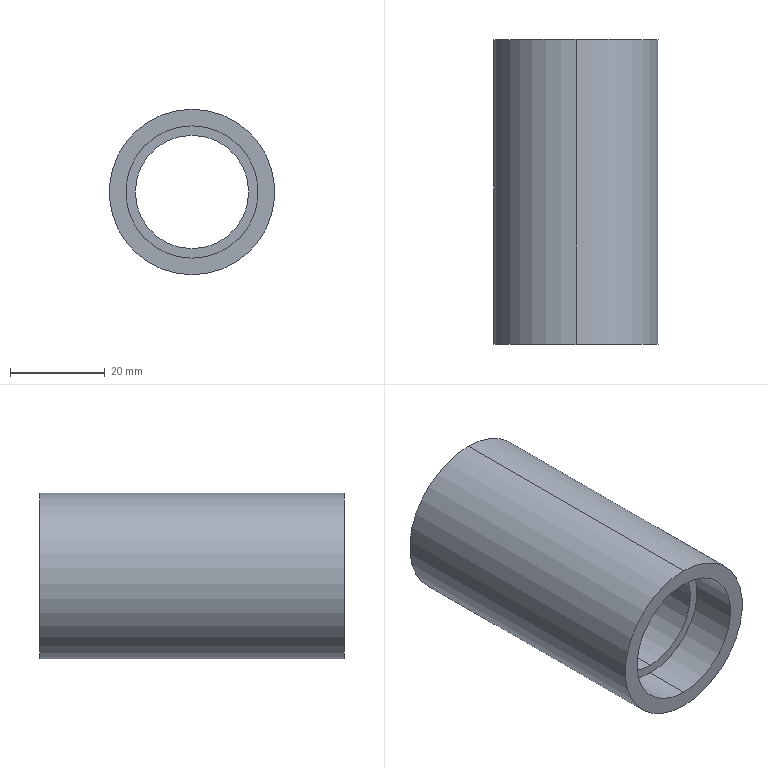Part | STEP file | ND25021-01-JDKM-15-TL | 1 solid | 12 faces | box 35 x 64.5 x 35 mm | volume 29610 mm3 | cylinder 8 | plane 4 | commonest cylinder face diameters 28 x4 24 x2 35 x2
STEP:
#1=CARTESIAN_POINT('',(0.,0.,0.));
#2=DIRECTION('',(0.,0.,1.));
#3=DIRECTION('',(1.,0.,0.));
#4=AXIS2_PLACEMENT_3D('',#1,#2,#3);
#5=CARTESIAN_POINT('',(0.,22.25,14.));
#6=VERTEX_POINT('',#5);
#7=CARTESIAN_POINT('',(0.,32.25,14.));
#8=VERTEX_POINT('',#7);
#9=CARTESIAN_POINT('',(0.,22.25,14.));
#10=DIRECTION('',(0.,1.,0.));
#11=VECTOR('',#10,1.);
#12=LINE('',#9,#11);
#13=CARTESIAN_POINT('',(0.,22.25,0.));
#14=DIRECTION('',(0.,1.,0.));
#15=DIRECTION('',(0.,0.,1.));
#16=AXIS2_PLACEMENT_3D('',#13,#14,#15);
#17=CYLINDRICAL_SURFACE('',#16,14.);
#18=CARTESIAN_POINT('',(6.283,0.));
#19=DIRECTION('',(0.,1.));
#20=VECTOR('',#19,1.);
#21=LINE('',#18,#20);
#22=(GEOMETRIC_REPRESENTATION_CONTEXT(2)PARAMETRIC_REPRESENTATION_CONTEXT()REPRESENTATION_CONTEXT('',''));
#23=DEFINITIONAL_REPRESENTATION('',(#21),#22);
#24=PCURVE('',#17,#23);
#25=CARTESIAN_POINT('',(0.,22.25,0.));
#26=DIRECTION('',(0.,1.,0.));
#27=DIRECTION('',(0.,0.,1.));
#28=AXIS2_PLACEMENT_3D('',#25,#26,#27);
#29=CYLINDRICAL_SURFACE('',#28,14.);
#30=CARTESIAN_POINT('',(0.,0.));
#31=DIRECTION('',(0.,1.));
#32=VECTOR('',#31,1.);
#33=LINE('',#30,#32);
#34=(GEOMETRIC_REPRESENTATION_CONTEXT(2)PARAMETRIC_REPRESENTATION_CONTEXT()REPRESENTATION_CONTEXT('',''));
#35=DEFINITIONAL_REPRESENTATION('',(#33),#34);
#36=PCURVE('',#29,#35);
#37=SURFACE_CURVE('',#12,(#24,#36),.PCURVE_S1.);
#38=EDGE_CURVE('',#6,#8,#37,.T.);
#39=ORIENTED_EDGE('',*,*,#38,.T.);
#40=CARTESIAN_POINT('',(0.,32.25,-14.));
#41=VERTEX_POINT('',#40);
#42=CARTESIAN_POINT('',(0.,32.25,0.));
#43=DIRECTION('',(0.,1.,0.));
#44=DIRECTION('',(0.,0.,1.));
#45=AXIS2_PLACEMENT_3D('',#42,#43,#44);
#46=CIRCLE('',#45,14.);
#47=CARTESIAN_POINT('',(0.,10.));
#48=DIRECTION('',(1.,0.));
#49=VECTOR('',#48,1.);
#50=LINE('',#47,#49);
#51=(GEOMETRIC_REPRESENTATION_CONTEXT(2)PARAMETRIC_REPRESENTATION_CONTEXT()REPRESENTATION_CONTEXT('',''));
#52=DEFINITIONAL_REPRESENTATION('',(#50),#51);
#53=PCURVE('',#17,#52);
#54=CARTESIAN_POINT('',(0.,32.25,0.));
#55=DIRECTION('',(0.,1.,0.));
#56=DIRECTION('',(0.,0.,1.));
#57=AXIS2_PLACEMENT_3D('',#54,#55,#56);
#58=PLANE('',#57);
#59=CARTESIAN_POINT('',(0.,0.));
#60=DIRECTION('',(1.,0.));
#61=AXIS2_PLACEMENT_2D('',#59,#60);
#62=CIRCLE('',#61,14.);
#63=(GEOMETRIC_REPRESENTATION_CONTEXT(2)PARAMETRIC_REPRESENTATION_CONTEXT()REPRESENTATION_CONTEXT('',''));
#64=DEFINITIONAL_REPRESENTATION('',(#62),#63);
#65=PCURVE('',#58,#64);
#66=SURFACE_CURVE('',#46,(#53,#65),.PCURVE_S1.);
#67=EDGE_CURVE('',#41,#8,#66,.T.);
#68=ORIENTED_EDGE('',*,*,#67,.F.);
#69=CARTESIAN_POINT('',(0.,22.25,-14.));
#70=VERTEX_POINT('',#69);
#71=CARTESIAN_POINT('',(0.,22.25,-14.));
#72=DIRECTION('',(0.,1.,0.));
#73=VECTOR('',#72,1.);
#74=LINE('',#71,#73);
#75=CARTESIAN_POINT('',(3.142,0.));
#76=DIRECTION('',(0.,1.));
#77=VECTOR('',#76,1.);
#78=LINE('',#75,#77);
#79=(GEOMETRIC_REPRESENTATION_CONTEXT(2)PARAMETRIC_REPRESENTATION_CONTEXT()REPRESENTATION_CONTEXT('',''));
#80=DEFINITIONAL_REPRESENTATION('',(#78),#79);
#81=PCURVE('',#17,#80);
#82=CARTESIAN_POINT('',(3.142,0.));
#83=DIRECTION('',(0.,1.));
#84=VECTOR('',#83,1.);
#85=LINE('',#82,#84);
#86=(GEOMETRIC_REPRESENTATION_CONTEXT(2)PARAMETRIC_REPRESENTATION_CONTEXT()REPRESENTATION_CONTEXT('',''));
#87=DEFINITIONAL_REPRESENTATION('',(#85),#86);
#88=PCURVE('',#29,#87);
#89=SURFACE_CURVE('',#74,(#81,#88),.PCURVE_S1.);
#90=EDGE_CURVE('',#70,#41,#89,.T.);
#91=ORIENTED_EDGE('',*,*,#90,.F.);
#92=CARTESIAN_POINT('',(0.,22.25,0.));
#93=DIRECTION('',(0.,1.,0.));
#94=DIRECTION('',(0.,0.,1.));
#95=AXIS2_PLACEMENT_3D('',#92,#93,#94);
#96=CIRCLE('',#95,14.);
#97=CARTESIAN_POINT('',(0.,0.));
#98=DIRECTION('',(1.,0.));
#99=VECTOR('',#98,1.);
#100=LINE('',#97,#99);
#101=(GEOMETRIC_REPRESENTATION_CONTEXT(2)PARAMETRIC_REPRESENTATION_CONTEXT()REPRESENTATION_CONTEXT('',''));
#102=DEFINITIONAL_REPRESENTATION('',(#100),#101);
#103=PCURVE('',#17,#102);
#104=CARTESIAN_POINT('',(0.,22.25,0.));
#105=DIRECTION('',(0.,1.,0.));
#106=DIRECTION('',(0.,0.,1.));
#107=AXIS2_PLACEMENT_3D('',#104,#105,#106);
#108=PLANE('',#107);
#109=CARTESIAN_POINT('',(0.,0.));
#110=DIRECTION('',(1.,0.));
#111=AXIS2_PLACEMENT_2D('',#109,#110);
#112=CIRCLE('',#111,14.);
#113=(GEOMETRIC_REPRESENTATION_CONTEXT(2)PARAMETRIC_REPRESENTATION_CONTEXT()REPRESENTATION_CONTEXT('',''));
#114=DEFINITIONAL_REPRESENTATION('',(#112),#113);
#115=PCURVE('',#108,#114);
#116=SURFACE_CURVE('',#96,(#103,#115),.PCURVE_S1.);
#117=EDGE_CURVE('',#70,#6,#116,.T.);
#118=ORIENTED_EDGE('',*,*,#117,.T.);
#119=EDGE_LOOP('',(#39,#68,#91,#118));
#120=FACE_BOUND('',#119,.F.);
#121=ADVANCED_FACE('',(#120),#17,.F.);
#122=CARTESIAN_POINT('',(0.,-22.25,-14.));
#123=VERTEX_POINT('',#122);
#124=CARTESIAN_POINT('',(0.,-32.25,-14.));
#125=VERTEX_POINT('',#124);
#126=CARTESIAN_POINT('',(0.,-22.25,-14.));
#127=DIRECTION('',(0.,-1.,0.));
#128=VECTOR('',#127,1.);
#129=LINE('',#126,#128);
#130=CARTESIAN_POINT('',(0.,-22.25,0.));
#131=DIRECTION('',(0.,-1.,0.));
#132=DIRECTION('',(0.,0.,-1.));
#133=AXIS2_PLACEMENT_3D('',#130,#131,#132);
#134=CYLINDRICAL_SURFACE('',#133,14.);
#135=CARTESIAN_POINT('',(6.283,0.));
#136=DIRECTION('',(0.,1.));
#137=VECTOR('',#136,1.);
#138=LINE('',#135,#137);
#139=(GEOMETRIC_REPRESENTATION_CONTEXT(2)PARAMETRIC_REPRESENTATION_CONTEXT()REPRESENTATION_CONTEXT('',''));
#140=DEFINITIONAL_REPRESENTATION('',(#138),#139);
#141=PCURVE('',#134,#140);
#142=CARTESIAN_POINT('',(0.,-22.25,0.));
#143=DIRECTION('',(0.,-1.,0.));
#144=DIRECTION('',(0.,0.,-1.));
#145=AXIS2_PLACEMENT_3D('',#142,#143,#144);
#146=CYLINDRICAL_SURFACE('',#145,14.);
#147=CARTESIAN_POINT('',(0.,0.));
#148=DIRECTION('',(0.,1.));
#149=VECTOR('',#148,1.);
#150=LINE('',#147,#149);
#151=(GEOMETRIC_REPRESENTATION_CONTEXT(2)PARAMETRIC_REPRESENTATION_CONTEXT()REPRESENTATION_CONTEXT('',''));
#152=DEFINITIONAL_REPRESENTATION('',(#150),#151);
#153=PCURVE('',#146,#152);
#154=SURFACE_CURVE('',#129,(#141,#153),.PCURVE_S1.);
#155=EDGE_CURVE('',#123,#125,#154,.T.);
#156=ORIENTED_EDGE('',*,*,#155,.T.);
#157=CARTESIAN_POINT('',(0.,-32.25,14.));
#158=VERTEX_POINT('',#157);
#159=CARTESIAN_POINT('',(0.,-32.25,0.));
#160=DIRECTION('',(0.,-1.,0.));
#161=DIRECTION('',(0.,0.,-1.));
#162=AXIS2_PLACEMENT_3D('',#159,#160,#161);
#163=CIRCLE('',#162,14.);
#164=CARTESIAN_POINT('',(0.,10.));
#165=DIRECTION('',(1.,0.));
#166=VECTOR('',#165,1.);
#167=LINE('',#164,#166);
#168=(GEOMETRIC_REPRESENTATION_CONTEXT(2)PARAMETRIC_REPRESENTATION_CONTEXT()REPRESENTATION_CONTEXT('',''));
#169=DEFINITIONAL_REPRESENTATION('',(#167),#168);
#170=PCURVE('',#134,#169);
#171=CARTESIAN_POINT('',(0.,-32.25,0.));
#172=DIRECTION('',(0.,1.,0.));
#173=DIRECTION('',(0.,0.,1.));
#174=AXIS2_PLACEMENT_3D('',#171,#172,#173);
#175=PLANE('',#174);
#176=CARTESIAN_POINT('',(-14.,0.));
#177=CARTESIAN_POINT('',(-14.,24.249));
#178=CARTESIAN_POINT('',(7.,12.124));
#179=CARTESIAN_POINT('',(28.,0.));
#180=CARTESIAN_POINT('',(7.,-12.124));
#181=CARTESIAN_POINT('',(-14.,-24.249));
#182=CARTESIAN_POINT('',(-14.,0.));
#183=(BOUNDED_CURVE()B_SPLINE_CURVE(2,(#176,#177,#178,#179,#180,#181,#182),.UNSPECIFIED.,.T.,.F.)B_SPLINE_CURVE_WITH_KNOTS((1,2,2,2,2,1),(-2.094,0.,2.094,4.189,6.283,8.378),.UNSPECIFIED.)CURVE()GEOMETRIC_REPRESENTATION_ITEM()RATIONAL_B_SPLINE_CURVE((1.,0.5,1.,0.5,1.,0.5,1.))REPRESENTATION_ITEM(''));
#184=(GEOMETRIC_REPRESENTATION_CONTEXT(2)PARAMETRIC_REPRESENTATION_CONTEXT()REPRESENTATION_CONTEXT('',''));
#185=DEFINITIONAL_REPRESENTATION('',(#183),#184);
#186=PCURVE('',#175,#185);
#187=SURFACE_CURVE('',#163,(#170,#186),.PCURVE_S1.);
#188=EDGE_CURVE('',#158,#125,#187,.T.);
#189=ORIENTED_EDGE('',*,*,#188,.F.);
#190=CARTESIAN_POINT('',(0.,-22.25,14.));
#191=VERTEX_POINT('',#190);
#192=CARTESIAN_POINT('',(0.,-22.25,14.));
#193=DIRECTION('',(0.,-1.,0.));
#194=VECTOR('',#193,1.);
#195=LINE('',#192,#194);
#196=CARTESIAN_POINT('',(3.142,0.));
#197=DIRECTION('',(0.,1.));
#198=VECTOR('',#197,1.);
#199=LINE('',#196,#198);
#200=(GEOMETRIC_REPRESENTATION_CONTEXT(2)PARAMETRIC_REPRESENTATION_CONTEXT()REPRESENTATION_CONTEXT('',''));
#201=DEFINITIONAL_REPRESENTATION('',(#199),#200);
#202=PCURVE('',#134,#201);
#203=CARTESIAN_POINT('',(3.142,0.));
#204=DIRECTION('',(0.,1.));
#205=VECTOR('',#204,1.);
#206=LINE('',#203,#205);
#207=(GEOMETRIC_REPRESENTATION_CONTEXT(2)PARAMETRIC_REPRESENTATION_CONTEXT()REPRESENTATION_CONTEXT('',''));
#208=DEFINITIONAL_REPRESENTATION('',(#206),#207);
#209=PCURVE('',#146,#208);
#210=SURFACE_CURVE('',#195,(#202,#209),.PCURVE_S1.);
#211=EDGE_CURVE('',#191,#158,#210,.T.);
#212=ORIENTED_EDGE('',*,*,#211,.F.);
#213=CARTESIAN_POINT('',(0.,-22.25,0.));
#214=DIRECTION('',(0.,-1.,0.));
#215=DIRECTION('',(0.,0.,-1.));
#216=AXIS2_PLACEMENT_3D('',#213,#214,#215);
#217=CIRCLE('',#216,14.);
#218=CARTESIAN_POINT('',(0.,0.));
#219=DIRECTION('',(1.,0.));
#220=VECTOR('',#219,1.);
#221=LINE('',#218,#220);
#222=(GEOMETRIC_REPRESENTATION_CONTEXT(2)PARAMETRIC_REPRESENTATION_CONTEXT()REPRESENTATION_CONTEXT('',''));
#223=DEFINITIONAL_REPRESENTATION('',(#221),#222);
#224=PCURVE('',#134,#223);
#225=CARTESIAN_POINT('',(0.,-22.25,0.));
#226=DIRECTION('',(0.,-1.,0.));
#227=DIRECTION('',(0.,0.,-1.));
#228=AXIS2_PLACEMENT_3D('',#225,#226,#227);
#229=PLANE('',#228);
#230=CARTESIAN_POINT('',(0.,0.));
#231=DIRECTION('',(1.,0.));
#232=AXIS2_PLACEMENT_2D('',#230,#231);
#233=CIRCLE('',#232,14.);
#234=(GEOMETRIC_REPRESENTATION_CONTEXT(2)PARAMETRIC_REPRESENTATION_CONTEXT()REPRESENTATION_CONTEXT('',''));
#235=DEFINITIONAL_REPRESENTATION('',(#233),#234);
#236=PCURVE('',#229,#235);
#237=SURFACE_CURVE('',#217,(#224,#236),.PCURVE_S1.);
#238=EDGE_CURVE('',#191,#123,#237,.T.);
#239=ORIENTED_EDGE('',*,*,#238,.T.);
#240=EDGE_LOOP('',(#156,#189,#212,#239));
#241=FACE_BOUND('',#240,.F.);
#242=ADVANCED_FACE('',(#241),#134,.F.);
#243=CARTESIAN_POINT('',(0.,32.25,17.5));
#244=VERTEX_POINT('',#243);
#245=CARTESIAN_POINT('',(0.,32.25,-17.5));
#246=VERTEX_POINT('',#245);
#247=CARTESIAN_POINT('',(0.,32.25,0.));
#248=DIRECTION('',(0.,1.,0.));
#249=DIRECTION('',(0.,0.,1.));
#250=AXIS2_PLACEMENT_3D('',#247,#248,#249);
#251=CIRCLE('',#250,17.5);
#252=CARTESIAN_POINT('',(0.,32.25,0.));
#253=DIRECTION('',(0.,-1.,0.));
#254=DIRECTION('',(0.,0.,-1.));
#255=AXIS2_PLACEMENT_3D('',#252,#253,#254);
#256=CYLINDRICAL_SURFACE('',#255,17.5);
#257=CARTESIAN_POINT('',(3.142,0.));
#258=DIRECTION('',(-1.,0.));
#259=VECTOR('',#258,1.);
#260=LINE('',#257,#259);
#261=(GEOMETRIC_REPRESENTATION_CONTEXT(2)PARAMETRIC_REPRESENTATION_CONTEXT()REPRESENTATION_CONTEXT('',''));
#262=DEFINITIONAL_REPRESENTATION('',(#260),#261);
#263=PCURVE('',#256,#262);
#264=CARTESIAN_POINT('',(0.,0.));
#265=DIRECTION('',(1.,0.));
#266=AXIS2_PLACEMENT_2D('',#264,#265);
#267=CIRCLE('',#266,17.5);
#268=(GEOMETRIC_REPRESENTATION_CONTEXT(2)PARAMETRIC_REPRESENTATION_CONTEXT()REPRESENTATION_CONTEXT('',''));
#269=DEFINITIONAL_REPRESENTATION('',(#267),#268);
#270=PCURVE('',#58,#269);
#271=SURFACE_CURVE('',#251,(#263,#270),.PCURVE_S1.);
#272=EDGE_CURVE('',#244,#246,#271,.T.);
#273=ORIENTED_EDGE('',*,*,#272,.F.);
#274=CARTESIAN_POINT('',(0.,-32.25,17.5));
#275=VERTEX_POINT('',#274);
#276=CARTESIAN_POINT('',(0.,32.25,17.5));
#277=DIRECTION('',(0.,-1.,0.));
#278=VECTOR('',#277,1.);
#279=LINE('',#276,#278);
#280=CARTESIAN_POINT('',(3.142,0.));
#281=DIRECTION('',(0.,1.));
#282=VECTOR('',#281,1.);
#283=LINE('',#280,#282);
#284=(GEOMETRIC_REPRESENTATION_CONTEXT(2)PARAMETRIC_REPRESENTATION_CONTEXT()REPRESENTATION_CONTEXT('',''));
#285=DEFINITIONAL_REPRESENTATION('',(#283),#284);
#286=PCURVE('',#256,#285);
#287=CARTESIAN_POINT('',(0.,32.25,0.));
#288=DIRECTION('',(0.,-1.,0.));
#289=DIRECTION('',(0.,0.,-1.));
#290=AXIS2_PLACEMENT_3D('',#287,#288,#289);
#291=CYLINDRICAL_SURFACE('',#290,17.5);
#292=CARTESIAN_POINT('',(3.142,0.));
#293=DIRECTION('',(0.,1.));
#294=VECTOR('',#293,1.);
#295=LINE('',#292,#294);
#296=(GEOMETRIC_REPRESENTATION_CONTEXT(2)PARAMETRIC_REPRESENTATION_CONTEXT()REPRESENTATION_CONTEXT('',''));
#297=DEFINITIONAL_REPRESENTATION('',(#295),#296);
#298=PCURVE('',#291,#297);
#299=SURFACE_CURVE('',#279,(#286,#298),.PCURVE_S1.);
#300=EDGE_CURVE('',#244,#275,#299,.T.);
#301=ORIENTED_EDGE('',*,*,#300,.T.);
#302=CARTESIAN_POINT('',(0.,-32.25,-17.5));
#303=VERTEX_POINT('',#302);
#304=CARTESIAN_POINT('',(0.,-32.25,0.));
#305=DIRECTION('',(0.,1.,0.));
#306=DIRECTION('',(0.,0.,1.));
#307=AXIS2_PLACEMENT_3D('',#304,#305,#306);
#308=CIRCLE('',#307,17.5);
#309=CARTESIAN_POINT('',(3.142,64.5));
#310=DIRECTION('',(-1.,0.));
#311=VECTOR('',#310,1.);
#312=LINE('',#309,#311);
#313=(GEOMETRIC_REPRESENTATION_CONTEXT(2)PARAMETRIC_REPRESENTATION_CONTEXT()REPRESENTATION_CONTEXT('',''));
#314=DEFINITIONAL_REPRESENTATION('',(#312),#313);
#315=PCURVE('',#256,#314);
#316=CARTESIAN_POINT('',(0.,0.));
#317=DIRECTION('',(1.,0.));
#318=AXIS2_PLACEMENT_2D('',#316,#317);
#319=CIRCLE('',#318,17.5);
#320=(GEOMETRIC_REPRESENTATION_CONTEXT(2)PARAMETRIC_REPRESENTATION_CONTEXT()REPRESENTATION_CONTEXT('',''));
#321=DEFINITIONAL_REPRESENTATION('',(#319),#320);
#322=PCURVE('',#175,#321);
#323=SURFACE_CURVE('',#308,(#315,#322),.PCURVE_S1.);
#324=EDGE_CURVE('',#275,#303,#323,.T.);
#325=ORIENTED_EDGE('',*,*,#324,.T.);
#326=CARTESIAN_POINT('',(0.,32.25,-17.5));
#327=DIRECTION('',(0.,-1.,0.));
#328=VECTOR('',#327,1.);
#329=LINE('',#326,#328);
#330=CARTESIAN_POINT('',(0.,0.));
#331=DIRECTION('',(0.,1.));
#332=VECTOR('',#331,1.);
#333=LINE('',#330,#332);
#334=(GEOMETRIC_REPRESENTATION_CONTEXT(2)PARAMETRIC_REPRESENTATION_CONTEXT()REPRESENTATION_CONTEXT('',''));
#335=DEFINITIONAL_REPRESENTATION('',(#333),#334);
#336=PCURVE('',#256,#335);
#337=CARTESIAN_POINT('',(6.283,0.));
#338=DIRECTION('',(0.,1.));
#339=VECTOR('',#338,1.);
#340=LINE('',#337,#339);
#341=(GEOMETRIC_REPRESENTATION_CONTEXT(2)PARAMETRIC_REPRESENTATION_CONTEXT()REPRESENTATION_CONTEXT('',''));
#342=DEFINITIONAL_REPRESENTATION('',(#340),#341);
#343=PCURVE('',#291,#342);
#344=SURFACE_CURVE('',#329,(#336,#343),.PCURVE_S1.);
#345=EDGE_CURVE('',#246,#303,#344,.T.);
#346=ORIENTED_EDGE('',*,*,#345,.F.);
#347=EDGE_LOOP('',(#273,#301,#325,#346));
#348=FACE_BOUND('',#347,.T.);
#349=ADVANCED_FACE('',(#348),#256,.T.);
#350=CARTESIAN_POINT('',(0.,22.25,-12.));
#351=VERTEX_POINT('',#350);
#352=CARTESIAN_POINT('',(0.,-22.25,-12.));
#353=VERTEX_POINT('',#352);
#354=CARTESIAN_POINT('',(0.,32.25,-12.));
#355=DIRECTION('',(0.,-1.,0.));
#356=VECTOR('',#355,1.);
#357=LINE('',#354,#356);
#358=CARTESIAN_POINT('',(0.,32.25,0.));
#359=DIRECTION('',(0.,-1.,0.));
#360=DIRECTION('',(0.,0.,-1.));
#361=AXIS2_PLACEMENT_3D('',#358,#359,#360);
#362=CYLINDRICAL_SURFACE('',#361,12.);
#363=CARTESIAN_POINT('',(6.283,0.));
#364=DIRECTION('',(0.,1.));
#365=VECTOR('',#364,1.);
#366=LINE('',#363,#365);
#367=(GEOMETRIC_REPRESENTATION_CONTEXT(2)PARAMETRIC_REPRESENTATION_CONTEXT()REPRESENTATION_CONTEXT('',''));
#368=DEFINITIONAL_REPRESENTATION('',(#366),#367);
#369=PCURVE('',#362,#368);
#370=CARTESIAN_POINT('',(0.,32.25,0.));
#371=DIRECTION('',(0.,-1.,0.));
#372=DIRECTION('',(0.,0.,-1.));
#373=AXIS2_PLACEMENT_3D('',#370,#371,#372);
#374=CYLINDRICAL_SURFACE('',#373,12.);
#375=CARTESIAN_POINT('',(0.,0.));
#376=DIRECTION('',(0.,1.));
#377=VECTOR('',#376,1.);
#378=LINE('',#375,#377);
#379=(GEOMETRIC_REPRESENTATION_CONTEXT(2)PARAMETRIC_REPRESENTATION_CONTEXT()REPRESENTATION_CONTEXT('',''));
#380=DEFINITIONAL_REPRESENTATION('',(#378),#379);
#381=PCURVE('',#374,#380);
#382=SURFACE_CURVE('',#357,(#369,#381),.PCURVE_S1.);
#383=EDGE_CURVE('',#351,#353,#382,.T.);
#384=ORIENTED_EDGE('',*,*,#383,.T.);
#385=CARTESIAN_POINT('',(0.,-22.25,12.));
#386=VERTEX_POINT('',#385);
#387=CARTESIAN_POINT('',(0.,-22.25,0.));
#388=DIRECTION('',(0.,1.,0.));
#389=DIRECTION('',(0.,0.,-1.));
#390=AXIS2_PLACEMENT_3D('',#387,#388,#389);
#391=CIRCLE('',#390,12.);
#392=CARTESIAN_POINT('',(6.283,54.5));
#393=DIRECTION('',(-1.,0.));
#394=VECTOR('',#393,1.);
#395=LINE('',#392,#394);
#396=(GEOMETRIC_REPRESENTATION_CONTEXT(2)PARAMETRIC_REPRESENTATION_CONTEXT()REPRESENTATION_CONTEXT('',''));
#397=DEFINITIONAL_REPRESENTATION('',(#395),#396);
#398=PCURVE('',#362,#397);
#399=CARTESIAN_POINT('',(12.,0.));
#400=CARTESIAN_POINT('',(12.,-20.785));
#401=CARTESIAN_POINT('',(-6.,-10.392));
#402=CARTESIAN_POINT('',(-24.,0.));
#403=CARTESIAN_POINT('',(-6.,10.392));
#404=CARTESIAN_POINT('',(12.,20.785));
#405=CARTESIAN_POINT('',(12.,0.));
#406=(BOUNDED_CURVE()B_SPLINE_CURVE(2,(#399,#400,#401,#402,#403,#404,#405),.UNSPECIFIED.,.T.,.F.)B_SPLINE_CURVE_WITH_KNOTS((1,2,2,2,2,1),(-2.094,0.,2.094,4.189,6.283,8.378),.UNSPECIFIED.)CURVE()GEOMETRIC_REPRESENTATION_ITEM()RATIONAL_B_SPLINE_CURVE((1.,0.5,1.,0.5,1.,0.5,1.))REPRESENTATION_ITEM(''));
#407=(GEOMETRIC_REPRESENTATION_CONTEXT(2)PARAMETRIC_REPRESENTATION_CONTEXT()REPRESENTATION_CONTEXT('',''));
#408=DEFINITIONAL_REPRESENTATION('',(#406),#407);
#409=PCURVE('',#229,#408);
#410=SURFACE_CURVE('',#391,(#398,#409),.PCURVE_S1.);
#411=EDGE_CURVE('',#353,#386,#410,.T.);
#412=ORIENTED_EDGE('',*,*,#411,.T.);
#413=CARTESIAN_POINT('',(0.,22.25,12.));
#414=VERTEX_POINT('',#413);
#415=CARTESIAN_POINT('',(0.,32.25,12.));
#416=DIRECTION('',(0.,-1.,0.));
#417=VECTOR('',#416,1.);
#418=LINE('',#415,#417);
#419=CARTESIAN_POINT('',(3.142,0.));
#420=DIRECTION('',(0.,1.));
#421=VECTOR('',#420,1.);
#422=LINE('',#419,#421);
#423=(GEOMETRIC_REPRESENTATION_CONTEXT(2)PARAMETRIC_REPRESENTATION_CONTEXT()REPRESENTATION_CONTEXT('',''));
#424=DEFINITIONAL_REPRESENTATION('',(#422),#423);
#425=PCURVE('',#362,#424);
#426=CARTESIAN_POINT('',(3.142,0.));
#427=DIRECTION('',(0.,1.));
#428=VECTOR('',#427,1.);
#429=LINE('',#426,#428);
#430=(GEOMETRIC_REPRESENTATION_CONTEXT(2)PARAMETRIC_REPRESENTATION_CONTEXT()REPRESENTATION_CONTEXT('',''));
#431=DEFINITIONAL_REPRESENTATION('',(#429),#430);
#432=PCURVE('',#374,#431);
#433=SURFACE_CURVE('',#418,(#425,#432),.PCURVE_S1.);
#434=EDGE_CURVE('',#414,#386,#433,.T.);
#435=ORIENTED_EDGE('',*,*,#434,.F.);
#436=CARTESIAN_POINT('',(0.,22.25,0.));
#437=DIRECTION('',(0.,-1.,0.));
#438=DIRECTION('',(0.,0.,1.));
#439=AXIS2_PLACEMENT_3D('',#436,#437,#438);
#440=CIRCLE('',#439,12.);
#441=CARTESIAN_POINT('',(3.142,10.));
#442=DIRECTION('',(1.,0.));
#443=VECTOR('',#442,1.);
#444=LINE('',#441,#443);
#445=(GEOMETRIC_REPRESENTATION_CONTEXT(2)PARAMETRIC_REPRESENTATION_CONTEXT()REPRESENTATION_CONTEXT('',''));
#446=DEFINITIONAL_REPRESENTATION('',(#444),#445);
#447=PCURVE('',#362,#446);
#448=CARTESIAN_POINT('',(12.,0.));
#449=CARTESIAN_POINT('',(12.,-20.785));
#450=CARTESIAN_POINT('',(-6.,-10.392));
#451=CARTESIAN_POINT('',(-24.,0.));
#452=CARTESIAN_POINT('',(-6.,10.392));
#453=CARTESIAN_POINT('',(12.,20.785));
#454=CARTESIAN_POINT('',(12.,0.));
#455=(BOUNDED_CURVE()B_SPLINE_CURVE(2,(#448,#449,#450,#451,#452,#453,#454),.UNSPECIFIED.,.T.,.F.)B_SPLINE_CURVE_WITH_KNOTS((1,2,2,2,2,1),(-2.094,0.,2.094,4.189,6.283,8.378),.UNSPECIFIED.)CURVE()GEOMETRIC_REPRESENTATION_ITEM()RATIONAL_B_SPLINE_CURVE((1.,0.5,1.,0.5,1.,0.5,1.))REPRESENTATION_ITEM(''));
#456=(GEOMETRIC_REPRESENTATION_CONTEXT(2)PARAMETRIC_REPRESENTATION_CONTEXT()REPRESENTATION_CONTEXT('',''));
#457=DEFINITIONAL_REPRESENTATION('',(#455),#456);
#458=PCURVE('',#108,#457);
#459=SURFACE_CURVE('',#440,(#447,#458),.PCURVE_S1.);
#460=EDGE_CURVE('',#414,#351,#459,.T.);
#461=ORIENTED_EDGE('',*,*,#460,.T.);
#462=EDGE_LOOP('',(#384,#412,#435,#461));
#463=FACE_BOUND('',#462,.F.);
#464=ADVANCED_FACE('',(#463),#362,.F.);
#465=CARTESIAN_POINT('',(0.,-22.25,0.));
#466=DIRECTION('',(0.,1.,0.));
#467=DIRECTION('',(0.,0.,-1.));
#468=AXIS2_PLACEMENT_3D('',#465,#466,#467);
#469=CIRCLE('',#468,12.);
#470=CARTESIAN_POINT('',(6.283,54.5));
#471=DIRECTION('',(-1.,0.));
#472=VECTOR('',#471,1.);
#473=LINE('',#470,#472);
#474=(GEOMETRIC_REPRESENTATION_CONTEXT(2)PARAMETRIC_REPRESENTATION_CONTEXT()REPRESENTATION_CONTEXT('',''));
#475=DEFINITIONAL_REPRESENTATION('',(#473),#474);
#476=PCURVE('',#374,#475);
#477=CARTESIAN_POINT('',(12.,0.));
#478=CARTESIAN_POINT('',(12.,-20.785));
#479=CARTESIAN_POINT('',(-6.,-10.392));
#480=CARTESIAN_POINT('',(-24.,0.));
#481=CARTESIAN_POINT('',(-6.,10.392));
#482=CARTESIAN_POINT('',(12.,20.785));
#483=CARTESIAN_POINT('',(12.,0.));
#484=(BOUNDED_CURVE()B_SPLINE_CURVE(2,(#477,#478,#479,#480,#481,#482,#483),.UNSPECIFIED.,.T.,.F.)B_SPLINE_CURVE_WITH_KNOTS((1,2,2,2,2,1),(-2.094,0.,2.094,4.189,6.283,8.378),.UNSPECIFIED.)CURVE()GEOMETRIC_REPRESENTATION_ITEM()RATIONAL_B_SPLINE_CURVE((1.,0.5,1.,0.5,1.,0.5,1.))REPRESENTATION_ITEM(''));
#485=(GEOMETRIC_REPRESENTATION_CONTEXT(2)PARAMETRIC_REPRESENTATION_CONTEXT()REPRESENTATION_CONTEXT('',''));
#486=DEFINITIONAL_REPRESENTATION('',(#484),#485);
#487=PCURVE('',#229,#486);
#488=SURFACE_CURVE('',#469,(#476,#487),.PCURVE_S1.);
#489=EDGE_CURVE('',#386,#353,#488,.T.);
#490=ORIENTED_EDGE('',*,*,#489,.T.);
#491=ORIENTED_EDGE('',*,*,#383,.F.);
#492=CARTESIAN_POINT('',(0.,22.25,0.));
#493=DIRECTION('',(0.,-1.,0.));
#494=DIRECTION('',(0.,0.,1.));
#495=AXIS2_PLACEMENT_3D('',#492,#493,#494);
#496=CIRCLE('',#495,12.);
#497=CARTESIAN_POINT('',(-3.142,10.));
#498=DIRECTION('',(1.,0.));
#499=VECTOR('',#498,1.);
#500=LINE('',#497,#499);
#501=(GEOMETRIC_REPRESENTATION_CONTEXT(2)PARAMETRIC_REPRESENTATION_CONTEXT()REPRESENTATION_CONTEXT('',''));
#502=DEFINITIONAL_REPRESENTATION('',(#500),#501);
#503=PCURVE('',#374,#502);
#504=CARTESIAN_POINT('',(12.,0.));
#505=CARTESIAN_POINT('',(12.,-20.785));
#506=CARTESIAN_POINT('',(-6.,-10.392));
#507=CARTESIAN_POINT('',(-24.,0.));
#508=CARTESIAN_POINT('',(-6.,10.392));
#509=CARTESIAN_POINT('',(12.,20.785));
#510=CARTESIAN_POINT('',(12.,0.));
#511=(BOUNDED_CURVE()B_SPLINE_CURVE(2,(#504,#505,#506,#507,#508,#509,#510),.UNSPECIFIED.,.T.,.F.)B_SPLINE_CURVE_WITH_KNOTS((1,2,2,2,2,1),(-2.094,0.,2.094,4.189,6.283,8.378),.UNSPECIFIED.)CURVE()GEOMETRIC_REPRESENTATION_ITEM()RATIONAL_B_SPLINE_CURVE((1.,0.5,1.,0.5,1.,0.5,1.))REPRESENTATION_ITEM(''));
#512=(GEOMETRIC_REPRESENTATION_CONTEXT(2)PARAMETRIC_REPRESENTATION_CONTEXT()REPRESENTATION_CONTEXT('',''));
#513=DEFINITIONAL_REPRESENTATION('',(#511),#512);
#514=PCURVE('',#108,#513);
#515=SURFACE_CURVE('',#496,(#503,#514),.PCURVE_S1.);
#516=EDGE_CURVE('',#351,#414,#515,.T.);
#517=ORIENTED_EDGE('',*,*,#516,.T.);
#518=ORIENTED_EDGE('',*,*,#434,.T.);
#519=EDGE_LOOP('',(#490,#491,#517,#518));
#520=FACE_BOUND('',#519,.F.);
#521=ADVANCED_FACE('',(#520),#374,.F.);
#522=ORIENTED_EDGE('',*,*,#300,.F.);
#523=CARTESIAN_POINT('',(0.,32.25,0.));
#524=DIRECTION('',(0.,1.,0.));
#525=DIRECTION('',(0.,0.,1.));
#526=AXIS2_PLACEMENT_3D('',#523,#524,#525);
#527=CIRCLE('',#526,17.5);
#528=CARTESIAN_POINT('',(9.425,0.));
#529=DIRECTION('',(-1.,0.));
#530=VECTOR('',#529,1.);
#531=LINE('',#528,#530);
#532=(GEOMETRIC_REPRESENTATION_CONTEXT(2)PARAMETRIC_REPRESENTATION_CONTEXT()REPRESENTATION_CONTEXT('',''));
#533=DEFINITIONAL_REPRESENTATION('',(#531),#532);
#534=PCURVE('',#291,#533);
#535=CARTESIAN_POINT('',(0.,0.));
#536=DIRECTION('',(1.,0.));
#537=AXIS2_PLACEMENT_2D('',#535,#536);
#538=CIRCLE('',#537,17.5);
#539=(GEOMETRIC_REPRESENTATION_CONTEXT(2)PARAMETRIC_REPRESENTATION_CONTEXT()REPRESENTATION_CONTEXT('',''));
#540=DEFINITIONAL_REPRESENTATION('',(#538),#539);
#541=PCURVE('',#58,#540);
#542=SURFACE_CURVE('',#527,(#534,#541),.PCURVE_S1.);
#543=EDGE_CURVE('',#246,#244,#542,.T.);
#544=ORIENTED_EDGE('',*,*,#543,.F.);
#545=ORIENTED_EDGE('',*,*,#345,.T.);
#546=CARTESIAN_POINT('',(0.,-32.25,0.));
#547=DIRECTION('',(0.,1.,0.));
#548=DIRECTION('',(0.,0.,1.));
#549=AXIS2_PLACEMENT_3D('',#546,#547,#548);
#550=CIRCLE('',#549,17.5);
#551=CARTESIAN_POINT('',(9.425,64.5));
#552=DIRECTION('',(-1.,0.));
#553=VECTOR('',#552,1.);
#554=LINE('',#551,#553);
#555=(GEOMETRIC_REPRESENTATION_CONTEXT(2)PARAMETRIC_REPRESENTATION_CONTEXT()REPRESENTATION_CONTEXT('',''));
#556=DEFINITIONAL_REPRESENTATION('',(#554),#555);
#557=PCURVE('',#291,#556);
#558=CARTESIAN_POINT('',(0.,0.));
#559=DIRECTION('',(1.,0.));
#560=AXIS2_PLACEMENT_2D('',#558,#559);
#561=CIRCLE('',#560,17.5);
#562=(GEOMETRIC_REPRESENTATION_CONTEXT(2)PARAMETRIC_REPRESENTATION_CONTEXT()REPRESENTATION_CONTEXT('',''));
#563=DEFINITIONAL_REPRESENTATION('',(#561),#562);
#564=PCURVE('',#175,#563);
#565=SURFACE_CURVE('',#550,(#557,#564),.PCURVE_S1.);
#566=EDGE_CURVE('',#303,#275,#565,.T.);
#567=ORIENTED_EDGE('',*,*,#566,.T.);
#568=EDGE_LOOP('',(#522,#544,#545,#567));
#569=FACE_BOUND('',#568,.T.);
#570=ADVANCED_FACE('',(#569),#291,.T.);
#571=CARTESIAN_POINT('',(0.,32.25,0.));
#572=DIRECTION('',(0.,1.,0.));
#573=DIRECTION('',(0.,0.,1.));
#574=AXIS2_PLACEMENT_3D('',#571,#572,#573);
#575=CIRCLE('',#574,14.);
#576=CARTESIAN_POINT('',(0.,0.));
#577=DIRECTION('',(1.,0.));
#578=AXIS2_PLACEMENT_2D('',#576,#577);
#579=CIRCLE('',#578,14.);
#580=(GEOMETRIC_REPRESENTATION_CONTEXT(2)PARAMETRIC_REPRESENTATION_CONTEXT()REPRESENTATION_CONTEXT('',''));
#581=DEFINITIONAL_REPRESENTATION('',(#579),#580);
#582=PCURVE('',#58,#581);
#583=CARTESIAN_POINT('',(0.,10.));
#584=DIRECTION('',(1.,0.));
#585=VECTOR('',#584,1.);
#586=LINE('',#583,#585);
#587=(GEOMETRIC_REPRESENTATION_CONTEXT(2)PARAMETRIC_REPRESENTATION_CONTEXT()REPRESENTATION_CONTEXT('',''));
#588=DEFINITIONAL_REPRESENTATION('',(#586),#587);
#589=PCURVE('',#29,#588);
#590=SURFACE_CURVE('',#575,(#582,#589),.PCURVE_S1.);
#591=EDGE_CURVE('',#8,#41,#590,.T.);
#592=ORIENTED_EDGE('',*,*,#591,.F.);
#593=ORIENTED_EDGE('',*,*,#67,.F.);
#594=EDGE_LOOP('',(#592,#593));
#595=FACE_BOUND('',#594,.T.);
#596=ORIENTED_EDGE('',*,*,#543,.T.);
#597=ORIENTED_EDGE('',*,*,#272,.T.);
#598=EDGE_LOOP('',(#596,#597));
#599=FACE_BOUND('',#598,.T.);
#600=ADVANCED_FACE('',(#595,#599),#58,.T.);
#601=CARTESIAN_POINT('',(0.,-32.25,0.));
#602=DIRECTION('',(0.,-1.,0.));
#603=DIRECTION('',(0.,0.,-1.));
#604=AXIS2_PLACEMENT_3D('',#601,#602,#603);
#605=CIRCLE('',#604,14.);
#606=CARTESIAN_POINT('',(-14.,0.));
#607=CARTESIAN_POINT('',(-14.,24.249));
#608=CARTESIAN_POINT('',(7.,12.124));
#609=CARTESIAN_POINT('',(28.,0.));
#610=CARTESIAN_POINT('',(7.,-12.124));
#611=CARTESIAN_POINT('',(-14.,-24.249));
#612=CARTESIAN_POINT('',(-14.,0.));
#613=(BOUNDED_CURVE()B_SPLINE_CURVE(2,(#606,#607,#608,#609,#610,#611,#612),.UNSPECIFIED.,.T.,.F.)B_SPLINE_CURVE_WITH_KNOTS((1,2,2,2,2,1),(-2.094,0.,2.094,4.189,6.283,8.378),.UNSPECIFIED.)CURVE()GEOMETRIC_REPRESENTATION_ITEM()RATIONAL_B_SPLINE_CURVE((1.,0.5,1.,0.5,1.,0.5,1.))REPRESENTATION_ITEM(''));
#614=(GEOMETRIC_REPRESENTATION_CONTEXT(2)PARAMETRIC_REPRESENTATION_CONTEXT()REPRESENTATION_CONTEXT('',''));
#615=DEFINITIONAL_REPRESENTATION('',(#613),#614);
#616=PCURVE('',#175,#615);
#617=CARTESIAN_POINT('',(0.,10.));
#618=DIRECTION('',(1.,0.));
#619=VECTOR('',#618,1.);
#620=LINE('',#617,#619);
#621=(GEOMETRIC_REPRESENTATION_CONTEXT(2)PARAMETRIC_REPRESENTATION_CONTEXT()REPRESENTATION_CONTEXT('',''));
#622=DEFINITIONAL_REPRESENTATION('',(#620),#621);
#623=PCURVE('',#146,#622);
#624=SURFACE_CURVE('',#605,(#616,#623),.PCURVE_S1.);
#625=EDGE_CURVE('',#125,#158,#624,.T.);
#626=ORIENTED_EDGE('',*,*,#625,.F.);
#627=ORIENTED_EDGE('',*,*,#188,.F.);
#628=EDGE_LOOP('',(#626,#627));
#629=FACE_BOUND('',#628,.T.);
#630=ORIENTED_EDGE('',*,*,#566,.F.);
#631=ORIENTED_EDGE('',*,*,#324,.F.);
#632=EDGE_LOOP('',(#630,#631));
#633=FACE_BOUND('',#632,.T.);
#634=ADVANCED_FACE('',(#629,#633),#175,.F.);
#635=CARTESIAN_POINT('',(0.,-22.25,0.));
#636=DIRECTION('',(0.,-1.,0.));
#637=DIRECTION('',(0.,0.,-1.));
#638=AXIS2_PLACEMENT_3D('',#635,#636,#637);
#639=CIRCLE('',#638,14.);
#640=CARTESIAN_POINT('',(0.,0.));
#641=DIRECTION('',(1.,0.));
#642=AXIS2_PLACEMENT_2D('',#640,#641);
#643=CIRCLE('',#642,14.);
#644=(GEOMETRIC_REPRESENTATION_CONTEXT(2)PARAMETRIC_REPRESENTATION_CONTEXT()REPRESENTATION_CONTEXT('',''));
#645=DEFINITIONAL_REPRESENTATION('',(#643),#644);
#646=PCURVE('',#229,#645);
#647=CARTESIAN_POINT('',(0.,0.));
#648=DIRECTION('',(1.,0.));
#649=VECTOR('',#648,1.);
#650=LINE('',#647,#649);
#651=(GEOMETRIC_REPRESENTATION_CONTEXT(2)PARAMETRIC_REPRESENTATION_CONTEXT()REPRESENTATION_CONTEXT('',''));
#652=DEFINITIONAL_REPRESENTATION('',(#650),#651);
#653=PCURVE('',#146,#652);
#654=SURFACE_CURVE('',#639,(#646,#653),.PCURVE_S1.);
#655=EDGE_CURVE('',#123,#191,#654,.T.);
#656=ORIENTED_EDGE('',*,*,#655,.T.);
#657=ORIENTED_EDGE('',*,*,#238,.T.);
#658=EDGE_LOOP('',(#656,#657));
#659=FACE_BOUND('',#658,.T.);
#660=ORIENTED_EDGE('',*,*,#411,.T.);
#661=ORIENTED_EDGE('',*,*,#489,.T.);
#662=EDGE_LOOP('',(#660,#661));
#663=FACE_BOUND('',#662,.T.);
#664=ADVANCED_FACE('',(#659,#663),#229,.T.);
#665=ORIENTED_EDGE('',*,*,#625,.F.);
#666=ORIENTED_EDGE('',*,*,#155,.F.);
#667=ORIENTED_EDGE('',*,*,#655,.T.);
#668=ORIENTED_EDGE('',*,*,#211,.T.);
#669=EDGE_LOOP('',(#665,#666,#667,#668));
#670=FACE_BOUND('',#669,.F.);
#671=ADVANCED_FACE('',(#670),#146,.F.);
#672=CARTESIAN_POINT('',(0.,22.25,0.));
#673=DIRECTION('',(0.,1.,0.));
#674=DIRECTION('',(0.,0.,1.));
#675=AXIS2_PLACEMENT_3D('',#672,#673,#674);
#676=CIRCLE('',#675,14.);
#677=CARTESIAN_POINT('',(0.,0.));
#678=DIRECTION('',(1.,0.));
#679=AXIS2_PLACEMENT_2D('',#677,#678);
#680=CIRCLE('',#679,14.);
#681=(GEOMETRIC_REPRESENTATION_CONTEXT(2)PARAMETRIC_REPRESENTATION_CONTEXT()REPRESENTATION_CONTEXT('',''));
#682=DEFINITIONAL_REPRESENTATION('',(#680),#681);
#683=PCURVE('',#108,#682);
#684=CARTESIAN_POINT('',(0.,0.));
#685=DIRECTION('',(1.,0.));
#686=VECTOR('',#685,1.);
#687=LINE('',#684,#686);
#688=(GEOMETRIC_REPRESENTATION_CONTEXT(2)PARAMETRIC_REPRESENTATION_CONTEXT()REPRESENTATION_CONTEXT('',''));
#689=DEFINITIONAL_REPRESENTATION('',(#687),#688);
#690=PCURVE('',#29,#689);
#691=SURFACE_CURVE('',#676,(#683,#690),.PCURVE_S1.);
#692=EDGE_CURVE('',#6,#70,#691,.T.);
#693=ORIENTED_EDGE('',*,*,#692,.T.);
#694=ORIENTED_EDGE('',*,*,#117,.T.);
#695=EDGE_LOOP('',(#693,#694));
#696=FACE_BOUND('',#695,.T.);
#697=ORIENTED_EDGE('',*,*,#516,.T.);
#698=ORIENTED_EDGE('',*,*,#460,.T.);
#699=EDGE_LOOP('',(#697,#698));
#700=FACE_BOUND('',#699,.T.);
#701=ADVANCED_FACE('',(#696,#700),#108,.T.);
#702=ORIENTED_EDGE('',*,*,#591,.F.);
#703=ORIENTED_EDGE('',*,*,#38,.F.);
#704=ORIENTED_EDGE('',*,*,#692,.T.);
#705=ORIENTED_EDGE('',*,*,#90,.T.);
#706=EDGE_LOOP('',(#702,#703,#704,#705));
#707=FACE_BOUND('',#706,.F.);
#708=ADVANCED_FACE('',(#707),#29,.F.);
#709=CLOSED_SHELL('',(#121,#242,#349,#464,#521,#570,#600,#634,#664,#671,#701,#708));
#710=MANIFOLD_SOLID_BREP('',#709);
#711=(LENGTH_UNIT()NAMED_UNIT(*)SI_UNIT(.MILLI.,.METRE.));
#712=UNCERTAINTY_MEASURE_WITH_UNIT(LENGTH_MEASURE(0.0000001),#711,'','');
#713=(NAMED_UNIT(*)PLANE_ANGLE_UNIT()SI_UNIT($,.RADIAN.));
#714=(NAMED_UNIT(*)SI_UNIT($,.STERADIAN.)SOLID_ANGLE_UNIT());
#715=(GEOMETRIC_REPRESENTATION_CONTEXT(3)GLOBAL_UNCERTAINTY_ASSIGNED_CONTEXT((#712))GLOBAL_UNIT_ASSIGNED_CONTEXT((#711,#713,#714))REPRESENTATION_CONTEXT('',''));
#716=ADVANCED_BREP_SHAPE_REPRESENTATION('',(#4,#710),#715);